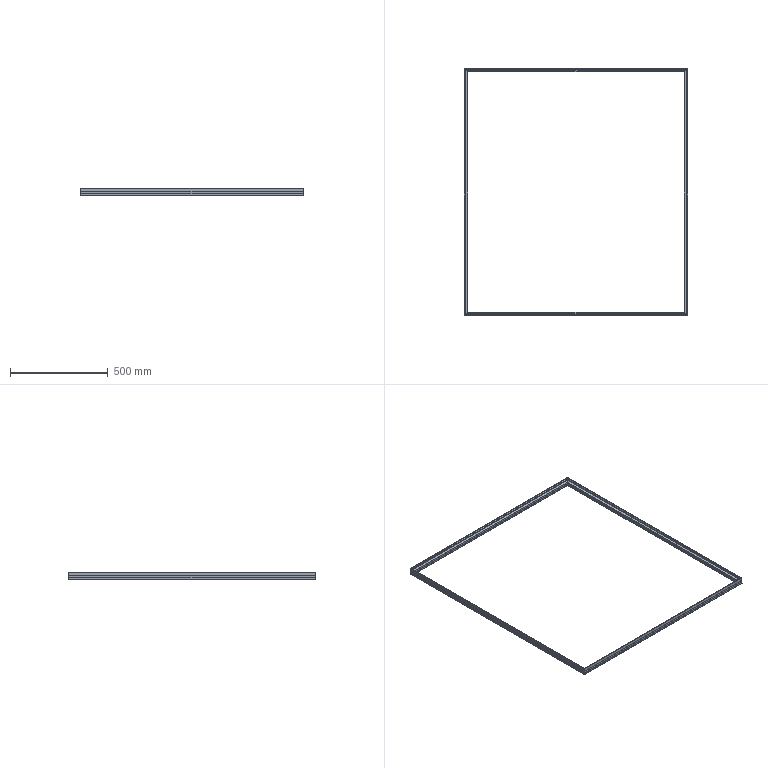Part | SolidWorks | features WeldMemberFeat 1, WeldmentFeature 1 | 4 solids | 96 faces | box 1140 x 1260 x 35 mm | volume 450066 mm3 | plane 96